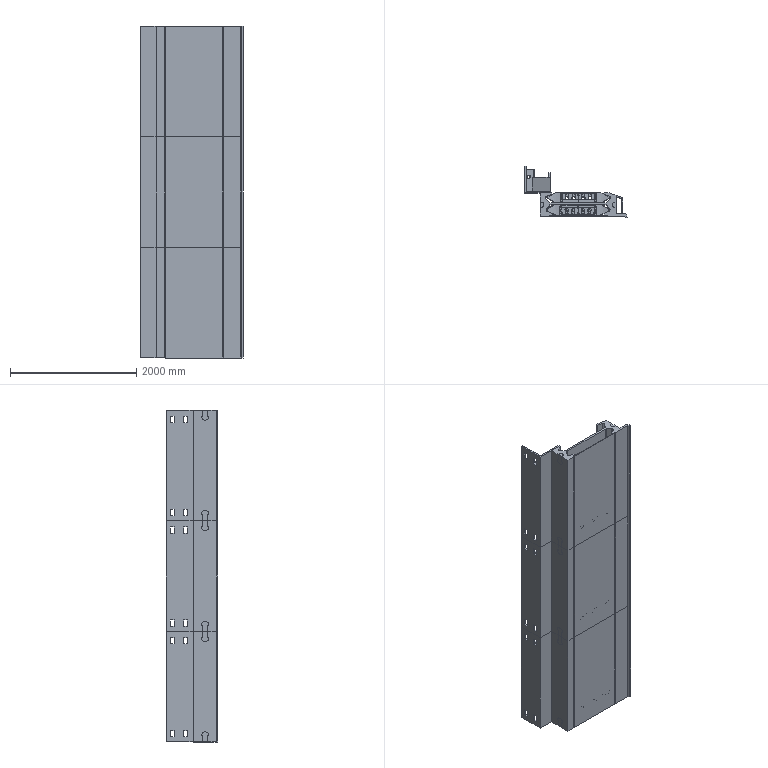Part | SolidWorks | 82 solids | 2682 faces | box 1628 x 811.488 x 5250 mm | volume 1041325350 mm3 | plane 1502 | cylinder 486 | spline 382 | cone 216 | torus 72 | sphere 24 | commonest cylinder face diameters 10 x150 80 x78 25 x42 33 x42 70 x42 50 x36